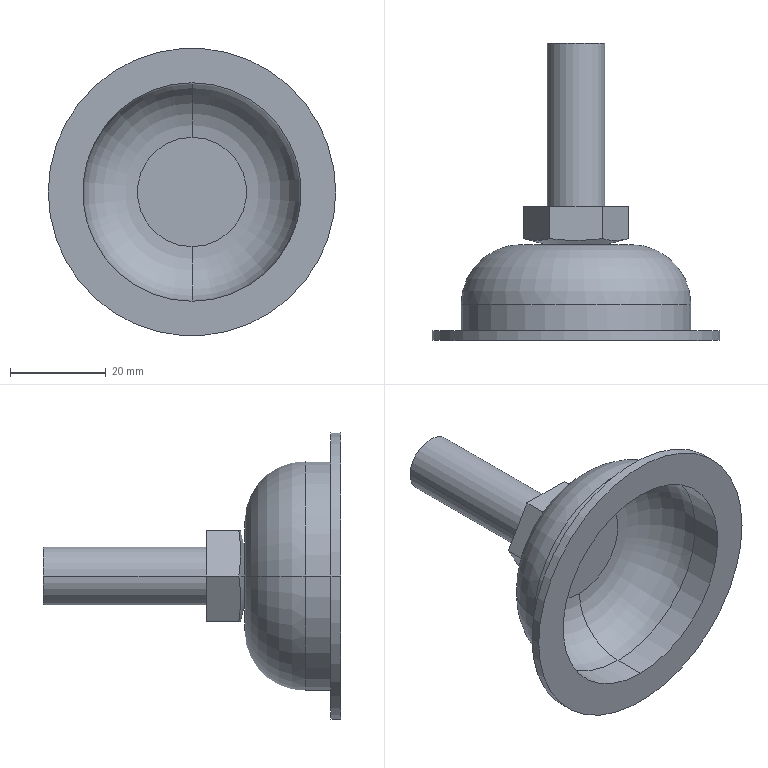Part | SolidWorks | features RefAxis 6, 3DProfileFeature 2, Revolution 2, Cut 1, ICE 1, RevCut 1 | 1 solid | 26 faces | box 60 x 62 x 60 mm | volume 14083 mm3 | plane 12 | cylinder 8 | torus 4 | cone 2 | commonest cylinder face diameters 12 x2 45.6 x2 48 x2 60 x2
STEP:
#1=CARTESIAN_POINT('',(0.,6.6,-22.8));
#2=VERTEX_POINT('',#1);
#3=CARTESIAN_POINT('',(0.,6.6,22.8));
#4=VERTEX_POINT('',#3);
#5=CARTESIAN_POINT('',(0.,6.6,0.));
#6=DIRECTION('',(0.,1.,0.));
#7=DIRECTION('',(0.,0.,1.));
#8=AXIS2_PLACEMENT_3D('',#5,#6,#7);
#9=CIRCLE('',#8,22.8);
#10=EDGE_CURVE('',#2,#4,#9,.T.);
#11=ORIENTED_EDGE('',*,*,#10,.F.);
#12=CARTESIAN_POINT('',(0.,18.,-11.4));
#13=VERTEX_POINT('',#12);
#14=CARTESIAN_POINT('',(0.,6.6,-11.4));
#15=DIRECTION('',(1.,0.,0.));
#16=DIRECTION('',(0.,0.,-1.));
#17=AXIS2_PLACEMENT_3D('',#14,#15,#16);
#18=CIRCLE('',#17,11.4);
#19=EDGE_CURVE('',#2,#13,#18,.T.);
#20=ORIENTED_EDGE('',*,*,#19,.T.);
#21=CARTESIAN_POINT('',(0.,18.,11.4));
#22=VERTEX_POINT('',#21);
#23=CARTESIAN_POINT('',(0.,18.,0.));
#24=DIRECTION('',(0.,1.,0.));
#25=DIRECTION('',(0.,0.,1.));
#26=AXIS2_PLACEMENT_3D('',#23,#24,#25);
#27=CIRCLE('',#26,11.4);
#28=EDGE_CURVE('',#13,#22,#27,.T.);
#29=ORIENTED_EDGE('',*,*,#28,.T.);
#30=CARTESIAN_POINT('',(0.,6.6,11.4));
#31=DIRECTION('',(-1.,0.,0.));
#32=DIRECTION('',(0.,0.,1.));
#33=AXIS2_PLACEMENT_3D('',#30,#31,#32);
#34=CIRCLE('',#33,11.4);
#35=EDGE_CURVE('',#4,#22,#34,.T.);
#36=ORIENTED_EDGE('',*,*,#35,.F.);
#37=EDGE_LOOP('',(#11,#20,#29,#36));
#38=FACE_OUTER_BOUND('',#37,.T.);
#39=CARTESIAN_POINT('',(0.,6.6,0.));
#40=DIRECTION('',(0.,1.,0.));
#41=DIRECTION('',(0.,0.,1.));
#42=AXIS2_PLACEMENT_3D('',#39,#40,#41);
#43=TOROIDAL_SURFACE('',#42,11.4,11.4);
#44=ADVANCED_FACE('',(#38),#43,.F.);
#45=CARTESIAN_POINT('',(0.,0.,22.8));
#46=VERTEX_POINT('',#45);
#47=CARTESIAN_POINT('',(0.,0.,-22.8));
#48=VERTEX_POINT('',#47);
#49=CARTESIAN_POINT('',(0.,0.,0.));
#50=DIRECTION('',(0.,-1.,0.));
#51=DIRECTION('',(-1.,0.,0.));
#52=AXIS2_PLACEMENT_3D('',#49,#50,#51);
#53=CIRCLE('',#52,22.8);
#54=EDGE_CURVE('',#46,#48,#53,.T.);
#55=ORIENTED_EDGE('',*,*,#54,.T.);
#56=CARTESIAN_POINT('',(0.,-1.,-22.8));
#57=DIRECTION('',(0.,1.,0.));
#58=VECTOR('',#57,1000.);
#59=LINE('',#56,#58);
#60=EDGE_CURVE('',#48,#2,#59,.T.);
#61=ORIENTED_EDGE('',*,*,#60,.T.);
#62=ORIENTED_EDGE('',*,*,#10,.T.);
#63=CARTESIAN_POINT('',(0.,-1.,22.8));
#64=DIRECTION('',(0.,1.,0.));
#65=VECTOR('',#64,1000.);
#66=LINE('',#63,#65);
#67=EDGE_CURVE('',#46,#4,#66,.T.);
#68=ORIENTED_EDGE('',*,*,#67,.F.);
#69=EDGE_LOOP('',(#55,#61,#62,#68));
#70=FACE_OUTER_BOUND('',#69,.T.);
#71=CARTESIAN_POINT('',(0.,-1.,0.));
#72=DIRECTION('',(0.,1.,0.));
#73=DIRECTION('',(0.,0.,1.));
#74=AXIS2_PLACEMENT_3D('',#71,#72,#73);
#75=CYLINDRICAL_SURFACE('',#74,22.8);
#76=ADVANCED_FACE('',(#70),#75,.F.);
#77=CARTESIAN_POINT('',(-30.,0.,0.));
#78=VERTEX_POINT('',#77);
#79=CARTESIAN_POINT('',(30.,0.,0.));
#80=VERTEX_POINT('',#79);
#81=CARTESIAN_POINT('',(0.,0.,0.));
#82=DIRECTION('',(0.,1.,0.));
#83=DIRECTION('',(-1.,0.,0.));
#84=AXIS2_PLACEMENT_3D('',#81,#82,#83);
#85=CIRCLE('',#84,30.);
#86=EDGE_CURVE('',#78,#80,#85,.T.);
#87=ORIENTED_EDGE('',*,*,#86,.T.);
#88=CARTESIAN_POINT('',(30.,2.,0.));
#89=VERTEX_POINT('',#88);
#90=CARTESIAN_POINT('',(30.,0.,0.));
#91=DIRECTION('',(0.,1.,0.));
#92=VECTOR('',#91,1000.);
#93=LINE('',#90,#92);
#94=EDGE_CURVE('',#80,#89,#93,.T.);
#95=ORIENTED_EDGE('',*,*,#94,.T.);
#96=CARTESIAN_POINT('',(-30.,2.,0.));
#97=VERTEX_POINT('',#96);
#98=CARTESIAN_POINT('',(0.,2.,0.));
#99=DIRECTION('',(0.,1.,0.));
#100=DIRECTION('',(-1.,0.,0.));
#101=AXIS2_PLACEMENT_3D('',#98,#99,#100);
#102=CIRCLE('',#101,30.);
#103=EDGE_CURVE('',#97,#89,#102,.T.);
#104=ORIENTED_EDGE('',*,*,#103,.F.);
#105=CARTESIAN_POINT('',(-30.,0.,0.));
#106=DIRECTION('',(0.,1.,0.));
#107=VECTOR('',#106,1000.);
#108=LINE('',#105,#107);
#109=EDGE_CURVE('',#78,#97,#108,.T.);
#110=ORIENTED_EDGE('',*,*,#109,.F.);
#111=EDGE_LOOP('',(#87,#95,#104,#110));
#112=FACE_OUTER_BOUND('',#111,.T.);
#113=CARTESIAN_POINT('',(0.,0.,0.));
#114=DIRECTION('',(0.,1.,0.));
#115=DIRECTION('',(-1.,0.,0.));
#116=AXIS2_PLACEMENT_3D('',#113,#114,#115);
#117=CYLINDRICAL_SURFACE('',#116,30.);
#118=ADVANCED_FACE('',(#112),#117,.T.);
#119=CARTESIAN_POINT('',(-24.,2.,0.));
#120=VERTEX_POINT('',#119);
#121=CARTESIAN_POINT('',(24.,2.,0.));
#122=VERTEX_POINT('',#121);
#123=CARTESIAN_POINT('',(0.,2.,0.));
#124=DIRECTION('',(0.,1.,0.));
#125=DIRECTION('',(-1.,0.,0.));
#126=AXIS2_PLACEMENT_3D('',#123,#124,#125);
#127=CIRCLE('',#126,24.);
#128=EDGE_CURVE('',#120,#122,#127,.T.);
#129=ORIENTED_EDGE('',*,*,#128,.T.);
#130=CARTESIAN_POINT('',(24.,7.4,0.));
#131=VERTEX_POINT('',#130);
#132=CARTESIAN_POINT('',(24.,0.,0.));
#133=DIRECTION('',(0.,1.,0.));
#134=VECTOR('',#133,1000.);
#135=LINE('',#132,#134);
#136=EDGE_CURVE('',#122,#131,#135,.T.);
#137=ORIENTED_EDGE('',*,*,#136,.T.);
#138=CARTESIAN_POINT('',(-24.,7.4,0.));
#139=VERTEX_POINT('',#138);
#140=CARTESIAN_POINT('',(0.,7.4,0.));
#141=DIRECTION('',(0.,1.,0.));
#142=DIRECTION('',(-1.,0.,0.));
#143=AXIS2_PLACEMENT_3D('',#140,#141,#142);
#144=CIRCLE('',#143,24.);
#145=EDGE_CURVE('',#139,#131,#144,.T.);
#146=ORIENTED_EDGE('',*,*,#145,.F.);
#147=CARTESIAN_POINT('',(-24.,0.,0.));
#148=DIRECTION('',(0.,1.,0.));
#149=VECTOR('',#148,1000.);
#150=LINE('',#147,#149);
#151=EDGE_CURVE('',#120,#139,#150,.T.);
#152=ORIENTED_EDGE('',*,*,#151,.F.);
#153=EDGE_LOOP('',(#129,#137,#146,#152));
#154=FACE_OUTER_BOUND('',#153,.T.);
#155=CARTESIAN_POINT('',(0.,0.,0.));
#156=DIRECTION('',(0.,1.,0.));
#157=DIRECTION('',(-1.,0.,0.));
#158=AXIS2_PLACEMENT_3D('',#155,#156,#157);
#159=CYLINDRICAL_SURFACE('',#158,24.);
#160=ADVANCED_FACE('',(#154),#159,.T.);
#161=ORIENTED_EDGE('',*,*,#145,.T.);
#162=CARTESIAN_POINT('',(11.4,20.,0.));
#163=VERTEX_POINT('',#162);
#164=CARTESIAN_POINT('',(11.4,7.4,0.));
#165=DIRECTION('',(0.,0.,1.));
#166=DIRECTION('',(1.,0.,0.));
#167=AXIS2_PLACEMENT_3D('',#164,#165,#166);
#168=CIRCLE('',#167,12.6);
#169=EDGE_CURVE('',#131,#163,#168,.T.);
#170=ORIENTED_EDGE('',*,*,#169,.T.);
#171=CARTESIAN_POINT('',(-11.4,20.,0.));
#172=VERTEX_POINT('',#171);
#173=CARTESIAN_POINT('',(0.,20.,0.));
#174=DIRECTION('',(0.,1.,0.));
#175=DIRECTION('',(-1.,0.,0.));
#176=AXIS2_PLACEMENT_3D('',#173,#174,#175);
#177=CIRCLE('',#176,11.4);
#178=EDGE_CURVE('',#172,#163,#177,.T.);
#179=ORIENTED_EDGE('',*,*,#178,.F.);
#180=CARTESIAN_POINT('',(-11.4,7.4,0.));
#181=DIRECTION('',(0.,0.,-1.));
#182=DIRECTION('',(-1.,0.,0.));
#183=AXIS2_PLACEMENT_3D('',#180,#181,#182);
#184=CIRCLE('',#183,12.6);
#185=EDGE_CURVE('',#139,#172,#184,.T.);
#186=ORIENTED_EDGE('',*,*,#185,.F.);
#187=EDGE_LOOP('',(#161,#170,#179,#186));
#188=FACE_OUTER_BOUND('',#187,.T.);
#189=CARTESIAN_POINT('',(0.,7.4,0.));
#190=DIRECTION('',(0.,1.,0.));
#191=DIRECTION('',(-1.,0.,0.));
#192=AXIS2_PLACEMENT_3D('',#189,#190,#191);
#193=TOROIDAL_SURFACE('',#192,11.4,12.6);
#194=ADVANCED_FACE('',(#188),#193,.T.);
#195=CARTESIAN_POINT('',(-6.,20.,0.));
#196=VERTEX_POINT('',#195);
#197=CARTESIAN_POINT('',(6.,20.,0.));
#198=VERTEX_POINT('',#197);
#199=CARTESIAN_POINT('',(0.,20.,0.));
#200=DIRECTION('',(0.,1.,0.));
#201=DIRECTION('',(-1.,0.,0.));
#202=AXIS2_PLACEMENT_3D('',#199,#200,#201);
#203=CIRCLE('',#202,6.);
#204=EDGE_CURVE('',#196,#198,#203,.T.);
#205=ORIENTED_EDGE('',*,*,#204,.T.);
#206=CARTESIAN_POINT('',(10.97,21.236,0.));
#207=VERTEX_POINT('',#206);
#208=CARTESIAN_POINT('',(6.,20.,0.));
#209=DIRECTION('',(0.9704,0.2414,0.));
#210=VECTOR('',#209,1000.);
#211=LINE('',#208,#210);
#212=EDGE_CURVE('',#198,#207,#211,.T.);
#213=ORIENTED_EDGE('',*,*,#212,.T.);
#214=CARTESIAN_POINT('',(5.485,21.236,9.5));
#215=VERTEX_POINT('',#214);
#216=CARTESIAN_POINT('',(10.97,21.236,0.));
#217=CARTESIAN_POINT('',(10.513,21.123,0.7917));
#218=CARTESIAN_POINT('',(10.056,21.03,1.583));
#219=CARTESIAN_POINT('',(9.141,20.904,3.167));
#220=CARTESIAN_POINT('',(8.227,20.837,4.75));
#221=CARTESIAN_POINT('',(7.313,20.904,6.333));
#222=CARTESIAN_POINT('',(6.399,21.03,7.917));
#223=CARTESIAN_POINT('',(5.942,21.123,8.708));
#224=CARTESIAN_POINT('',(5.485,21.236,9.5));
#225=B_SPLINE_CURVE_WITH_KNOTS('',3,(#216,#217,#218,#219,#220,#221,#222,#223,#224),.UNSPECIFIED.,.F.,.F.,(4,2,1,2,4),(0.000000231,0.002743,0.005485,0.008227,0.01097),.UNSPECIFIED.);
#226=EDGE_CURVE('',#207,#215,#225,.T.);
#227=ORIENTED_EDGE('',*,*,#226,.T.);
#228=CARTESIAN_POINT('',(-5.485,21.236,9.5));
#229=VERTEX_POINT('',#228);
#230=CARTESIAN_POINT('',(5.485,21.236,9.5));
#231=CARTESIAN_POINT('',(3.662,21.01,9.5));
#232=CARTESIAN_POINT('',(1.837,20.871,9.5));
#233=CARTESIAN_POINT('',(-0.9062,20.871,9.5));
#234=CARTESIAN_POINT('',(-1.822,20.904,9.5));
#235=CARTESIAN_POINT('',(-3.654,21.03,9.5));
#236=CARTESIAN_POINT('',(-4.572,21.123,9.5));
#237=CARTESIAN_POINT('',(-5.485,21.236,9.5));
#238=B_SPLINE_CURVE_WITH_KNOTS('',3,(#230,#231,#232,#233,#234,#235,#236,#237),.UNSPECIFIED.,.F.,.F.,(4,2,2,4),(0.02128,0.02679,0.02955,0.0323),.UNSPECIFIED.);
#239=EDGE_CURVE('',#215,#229,#238,.T.);
#240=ORIENTED_EDGE('',*,*,#239,.T.);
#241=CARTESIAN_POINT('',(-10.97,21.236,0.));
#242=VERTEX_POINT('',#241);
#243=CARTESIAN_POINT('',(-5.485,21.236,9.5));
#244=CARTESIAN_POINT('',(-5.942,21.123,8.708));
#245=CARTESIAN_POINT('',(-6.399,21.03,7.917));
#246=CARTESIAN_POINT('',(-7.313,20.904,6.333));
#247=CARTESIAN_POINT('',(-8.227,20.837,4.75));
#248=CARTESIAN_POINT('',(-9.141,20.904,3.167));
#249=CARTESIAN_POINT('',(-10.056,21.03,1.583));
#250=CARTESIAN_POINT('',(-10.513,21.123,0.7917));
#251=CARTESIAN_POINT('',(-10.97,21.236,0.));
#252=B_SPLINE_CURVE_WITH_KNOTS('',3,(#243,#244,#245,#246,#247,#248,#249,#250,#251),.UNSPECIFIED.,.F.,.F.,(4,2,1,2,4),(0.000000231,0.002743,0.005485,0.008227,0.01097),.UNSPECIFIED.);
#253=EDGE_CURVE('',#229,#242,#252,.T.);
#254=ORIENTED_EDGE('',*,*,#253,.T.);
#255=CARTESIAN_POINT('',(-6.,20.,0.));
#256=DIRECTION('',(-0.9704,0.2414,0.));
#257=VECTOR('',#256,1000.);
#258=LINE('',#255,#257);
#259=EDGE_CURVE('',#196,#242,#258,.T.);
#260=ORIENTED_EDGE('',*,*,#259,.F.);
#261=EDGE_LOOP('',(#205,#213,#227,#240,#254,#260));
#262=FACE_OUTER_BOUND('',#261,.T.);
#263=CARTESIAN_POINT('',(0.,20.,0.));
#264=DIRECTION('',(0.,1.,0.));
#265=DIRECTION('',(-1.,0.,0.));
#266=AXIS2_PLACEMENT_3D('',#263,#264,#265);
#267=CONICAL_SURFACE('',#266,6.,1.327);
#268=ADVANCED_FACE('',(#262),#267,.T.);
#269=CARTESIAN_POINT('',(-6.,28.,0.));
#270=VERTEX_POINT('',#269);
#271=CARTESIAN_POINT('',(6.,28.,0.));
#272=VERTEX_POINT('',#271);
#273=CARTESIAN_POINT('',(0.,28.,0.));
#274=DIRECTION('',(0.,1.,0.));
#275=DIRECTION('',(1.,0.,0.));
#276=AXIS2_PLACEMENT_3D('',#273,#274,#275);
#277=CIRCLE('',#276,6.);
#278=EDGE_CURVE('',#270,#272,#277,.T.);
#279=ORIENTED_EDGE('',*,*,#278,.T.);
#280=CARTESIAN_POINT('',(6.,62.,0.));
#281=VERTEX_POINT('',#280);
#282=CARTESIAN_POINT('',(6.,28.,0.));
#283=DIRECTION('',(0.,1.,0.));
#284=VECTOR('',#283,1000.);
#285=LINE('',#282,#284);
#286=EDGE_CURVE('',#272,#281,#285,.T.);
#287=ORIENTED_EDGE('',*,*,#286,.T.);
#288=CARTESIAN_POINT('',(-6.,62.,0.));
#289=VERTEX_POINT('',#288);
#290=CARTESIAN_POINT('',(0.,62.,0.));
#291=DIRECTION('',(0.,1.,0.));
#292=DIRECTION('',(-1.,0.,0.));
#293=AXIS2_PLACEMENT_3D('',#290,#291,#292);
#294=CIRCLE('',#293,6.);
#295=EDGE_CURVE('',#289,#281,#294,.T.);
#296=ORIENTED_EDGE('',*,*,#295,.F.);
#297=CARTESIAN_POINT('',(-6.,28.,0.));
#298=DIRECTION('',(0.,1.,0.));
#299=VECTOR('',#298,1000.);
#300=LINE('',#297,#299);
#301=EDGE_CURVE('',#270,#289,#300,.T.);
#302=ORIENTED_EDGE('',*,*,#301,.F.);
#303=EDGE_LOOP('',(#279,#287,#296,#302));
#304=FACE_OUTER_BOUND('',#303,.T.);
#305=CARTESIAN_POINT('',(0.,28.,0.));
#306=DIRECTION('',(0.,1.,0.));
#307=DIRECTION('',(-1.,0.,0.));
#308=AXIS2_PLACEMENT_3D('',#305,#306,#307);
#309=CYLINDRICAL_SURFACE('',#308,6.);
#310=ADVANCED_FACE('',(#304),#309,.T.);
#311=ORIENTED_EDGE('',*,*,#286,.F.);
#312=CARTESIAN_POINT('',(0.,28.,0.));
#313=DIRECTION('',(0.,1.,0.));
#314=DIRECTION('',(1.,0.,0.));
#315=AXIS2_PLACEMENT_3D('',#312,#313,#314);
#316=CIRCLE('',#315,6.);
#317=EDGE_CURVE('',#272,#270,#316,.T.);
#318=ORIENTED_EDGE('',*,*,#317,.T.);
#319=ORIENTED_EDGE('',*,*,#301,.T.);
#320=CARTESIAN_POINT('',(0.,62.,0.));
#321=DIRECTION('',(0.,1.,0.));
#322=DIRECTION('',(-1.,0.,0.));
#323=AXIS2_PLACEMENT_3D('',#320,#321,#322);
#324=CIRCLE('',#323,6.);
#325=EDGE_CURVE('',#281,#289,#324,.T.);
#326=ORIENTED_EDGE('',*,*,#325,.F.);
#327=EDGE_LOOP('',(#311,#318,#319,#326));
#328=FACE_OUTER_BOUND('',#327,.T.);
#329=CARTESIAN_POINT('',(0.,28.,0.));
#330=DIRECTION('',(0.,1.,0.));
#331=DIRECTION('',(-1.,0.,0.));
#332=AXIS2_PLACEMENT_3D('',#329,#330,#331);
#333=CYLINDRICAL_SURFACE('',#332,6.);
#334=ADVANCED_FACE('',(#328),#333,.T.);
#335=ORIENTED_EDGE('',*,*,#86,.F.);
#336=CARTESIAN_POINT('',(0.,0.,0.));
#337=DIRECTION('',(0.,1.,0.));
#338=DIRECTION('',(-1.,0.,0.));
#339=AXIS2_PLACEMENT_3D('',#336,#337,#338);
#340=CIRCLE('',#339,30.);
#341=EDGE_CURVE('',#80,#78,#340,.T.);
#342=ORIENTED_EDGE('',*,*,#341,.F.);
#343=EDGE_LOOP('',(#335,#342));
#344=FACE_OUTER_BOUND('',#343,.T.);
#345=ORIENTED_EDGE('',*,*,#54,.F.);
#346=CARTESIAN_POINT('',(0.,0.,0.));
#347=DIRECTION('',(0.,-1.,0.));
#348=DIRECTION('',(-1.,0.,0.));
#349=AXIS2_PLACEMENT_3D('',#346,#347,#348);
#350=CIRCLE('',#349,22.8);
#351=EDGE_CURVE('',#48,#46,#350,.T.);
#352=ORIENTED_EDGE('',*,*,#351,.F.);
#353=EDGE_LOOP('',(#345,#352));
#354=FACE_BOUND('',#353,.T.);
#355=CARTESIAN_POINT('',(30.,0.,0.));
#356=DIRECTION('',(0.,1.,0.));
#357=DIRECTION('',(-1.,0.,0.));
#358=AXIS2_PLACEMENT_3D('',#355,#356,#357);
#359=PLANE('',#358);
#360=ADVANCED_FACE('',(#344,#354),#359,.F.);
#361=ORIENTED_EDGE('',*,*,#212,.F.);
#362=CARTESIAN_POINT('',(0.,20.,0.));
#363=DIRECTION('',(0.,1.,0.));
#364=DIRECTION('',(-1.,0.,0.));
#365=AXIS2_PLACEMENT_3D('',#362,#363,#364);
#366=CIRCLE('',#365,6.);
#367=EDGE_CURVE('',#198,#196,#366,.T.);
#368=ORIENTED_EDGE('',*,*,#367,.T.);
#369=ORIENTED_EDGE('',*,*,#259,.T.);
#370=CARTESIAN_POINT('',(-5.485,21.236,-9.5));
#371=VERTEX_POINT('',#370);
#372=CARTESIAN_POINT('',(-10.97,21.236,0.));
#373=CARTESIAN_POINT('',(-10.513,21.123,-0.7917));
#374=CARTESIAN_POINT('',(-10.056,21.03,-1.583));
#375=CARTESIAN_POINT('',(-9.141,20.904,-3.167));
#376=CARTESIAN_POINT('',(-8.227,20.837,-4.75));
#377=CARTESIAN_POINT('',(-7.313,20.904,-6.333));
#378=CARTESIAN_POINT('',(-6.399,21.03,-7.917));
#379=CARTESIAN_POINT('',(-5.942,21.123,-8.708));
#380=CARTESIAN_POINT('',(-5.485,21.236,-9.5));
#381=B_SPLINE_CURVE_WITH_KNOTS('',3,(#372,#373,#374,#375,#376,#377,#378,#379,#380),.UNSPECIFIED.,.F.,.F.,(4,2,1,2,4),(0.000000231,0.002743,0.005485,0.008227,0.01097),.UNSPECIFIED.);
#382=EDGE_CURVE('',#242,#371,#381,.T.);
#383=ORIENTED_EDGE('',*,*,#382,.T.);
#384=CARTESIAN_POINT('',(5.485,21.236,-9.5));
#385=VERTEX_POINT('',#384);
#386=CARTESIAN_POINT('',(-5.485,21.236,-9.5));
#387=CARTESIAN_POINT('',(-4.572,21.123,-9.5));
#388=CARTESIAN_POINT('',(-3.654,21.03,-9.5));
#389=CARTESIAN_POINT('',(-1.822,20.904,-9.5));
#390=CARTESIAN_POINT('',(-0.9062,20.871,-9.5));
#391=CARTESIAN_POINT('',(1.837,20.871,-9.5));
#392=CARTESIAN_POINT('',(3.662,21.01,-9.5));
#393=CARTESIAN_POINT('',(5.485,21.236,-9.5));
#394=B_SPLINE_CURVE_WITH_KNOTS('',3,(#386,#387,#388,#389,#390,#391,#392,#393),.UNSPECIFIED.,.F.,.F.,(4,2,2,4),(0.009106,0.01186,0.01462,0.02014),.UNSPECIFIED.);
#395=EDGE_CURVE('',#371,#385,#394,.T.);
#396=ORIENTED_EDGE('',*,*,#395,.T.);
#397=CARTESIAN_POINT('',(5.485,21.236,-9.5));
#398=CARTESIAN_POINT('',(5.942,21.123,-8.708));
#399=CARTESIAN_POINT('',(6.399,21.03,-7.917));
#400=CARTESIAN_POINT('',(7.313,20.904,-6.333));
#401=CARTESIAN_POINT('',(8.227,20.837,-4.75));
#402=CARTESIAN_POINT('',(9.141,20.904,-3.167));
#403=CARTESIAN_POINT('',(10.056,21.03,-1.583));
#404=CARTESIAN_POINT('',(10.513,21.123,-0.7917));
#405=CARTESIAN_POINT('',(10.97,21.236,0.));
#406=B_SPLINE_CURVE_WITH_KNOTS('',3,(#397,#398,#399,#400,#401,#402,#403,#404,#405),.UNSPECIFIED.,.F.,.F.,(4,2,1,2,4),(0.000000231,0.002743,0.005485,0.008227,0.01097),.UNSPECIFIED.);
#407=EDGE_CURVE('',#385,#207,#406,.T.);
#408=ORIENTED_EDGE('',*,*,#407,.T.);
#409=EDGE_LOOP('',(#361,#368,#369,#383,#396,#408));
#410=FACE_OUTER_BOUND('',#409,.T.);
#411=CARTESIAN_POINT('',(0.,20.,0.));
#412=DIRECTION('',(0.,1.,0.));
#413=DIRECTION('',(-1.,0.,0.));
#414=AXIS2_PLACEMENT_3D('',#411,#412,#413);
#415=CONICAL_SURFACE('',#414,6.,1.327);
#416=ADVANCED_FACE('',(#410),#415,.T.);
#417=ORIENTED_EDGE('',*,*,#204,.F.);
#418=ORIENTED_EDGE('',*,*,#367,.F.);
#419=EDGE_LOOP('',(#417,#418));
#420=FACE_BOUND('',#419,.T.);
#421=ORIENTED_EDGE('',*,*,#178,.T.);
#422=CARTESIAN_POINT('',(0.,20.,0.));
#423=DIRECTION('',(0.,1.,0.));
#424=DIRECTION('',(-1.,0.,0.));
#425=AXIS2_PLACEMENT_3D('',#422,#423,#424);
#426=CIRCLE('',#425,11.4);
#427=EDGE_CURVE('',#163,#172,#426,.T.);
#428=ORIENTED_EDGE('',*,*,#427,.T.);
#429=EDGE_LOOP('',(#421,#428));
#430=FACE_OUTER_BOUND('',#429,.T.);
#431=CARTESIAN_POINT('',(6.,20.,0.));
#432=DIRECTION('',(0.,-1.,0.));
#433=DIRECTION('',(1.,0.,0.));
#434=AXIS2_PLACEMENT_3D('',#431,#432,#433);
#435=PLANE('',#434);
#436=ADVANCED_FACE('',(#420,#430),#435,.F.);
#437=ORIENTED_EDGE('',*,*,#169,.F.);
#438=CARTESIAN_POINT('',(0.,7.4,0.));
#439=DIRECTION('',(0.,1.,0.));
#440=DIRECTION('',(-1.,0.,0.));
#441=AXIS2_PLACEMENT_3D('',#438,#439,#440);
#442=CIRCLE('',#441,24.);
#443=EDGE_CURVE('',#131,#139,#442,.T.);
#444=ORIENTED_EDGE('',*,*,#443,.T.);
#445=ORIENTED_EDGE('',*,*,#185,.T.);
#446=ORIENTED_EDGE('',*,*,#427,.F.);
#447=EDGE_LOOP('',(#437,#444,#445,#446));
#448=FACE_OUTER_BOUND('',#447,.T.);
#449=CARTESIAN_POINT('',(0.,7.4,0.));
#450=DIRECTION('',(0.,1.,0.));
#451=DIRECTION('',(-1.,0.,0.));
#452=AXIS2_PLACEMENT_3D('',#449,#450,#451);
#453=TOROIDAL_SURFACE('',#452,11.4,12.6);
#454=ADVANCED_FACE('',(#448),#453,.T.);
#455=ORIENTED_EDGE('',*,*,#136,.F.);
#456=CARTESIAN_POINT('',(0.,2.,0.));
#457=DIRECTION('',(0.,1.,0.));
#458=DIRECTION('',(-1.,0.,0.));
#459=AXIS2_PLACEMENT_3D('',#456,#457,#458);
#460=CIRCLE('',#459,24.);
#461=EDGE_CURVE('',#122,#120,#460,.T.);
#462=ORIENTED_EDGE('',*,*,#461,.T.);
#463=ORIENTED_EDGE('',*,*,#151,.T.);
#464=ORIENTED_EDGE('',*,*,#443,.F.);
#465=EDGE_LOOP('',(#455,#462,#463,#464));
#466=FACE_OUTER_BOUND('',#465,.T.);
#467=CARTESIAN_POINT('',(0.,0.,0.));
#468=DIRECTION('',(0.,1.,0.));
#469=DIRECTION('',(-1.,0.,0.));
#470=AXIS2_PLACEMENT_3D('',#467,#468,#469);
#471=CYLINDRICAL_SURFACE('',#470,24.);
#472=ADVANCED_FACE('',(#466),#471,.T.);
#473=ORIENTED_EDGE('',*,*,#128,.F.);
#474=ORIENTED_EDGE('',*,*,#461,.F.);
#475=EDGE_LOOP('',(#473,#474));
#476=FACE_BOUND('',#475,.T.);
#477=ORIENTED_EDGE('',*,*,#103,.T.);
#478=CARTESIAN_POINT('',(0.,2.,0.));
#479=DIRECTION('',(0.,1.,0.));
#480=DIRECTION('',(-1.,0.,0.));
#481=AXIS2_PLACEMENT_3D('',#478,#479,#480);
#482=CIRCLE('',#481,30.);
#483=EDGE_CURVE('',#89,#97,#482,.T.);
#484=ORIENTED_EDGE('',*,*,#483,.T.);
#485=EDGE_LOOP('',(#477,#484));
#486=FACE_OUTER_BOUND('',#485,.T.);
#487=CARTESIAN_POINT('',(24.,2.,0.));
#488=DIRECTION('',(0.,-1.,0.));
#489=DIRECTION('',(1.,0.,0.));
#490=AXIS2_PLACEMENT_3D('',#487,#488,#489);
#491=PLANE('',#490);
#492=ADVANCED_FACE('',(#476,#486),#491,.F.);
#493=ORIENTED_EDGE('',*,*,#94,.F.);
#494=ORIENTED_EDGE('',*,*,#341,.T.);
#495=ORIENTED_EDGE('',*,*,#109,.T.);
#496=ORIENTED_EDGE('',*,*,#483,.F.);
#497=EDGE_LOOP('',(#493,#494,#495,#496));
#498=FACE_OUTER_BOUND('',#497,.T.);
#499=CARTESIAN_POINT('',(0.,0.,0.));
#500=DIRECTION('',(0.,1.,0.));
#501=DIRECTION('',(-1.,0.,0.));
#502=AXIS2_PLACEMENT_3D('',#499,#500,#501);
#503=CYLINDRICAL_SURFACE('',#502,30.);
#504=ADVANCED_FACE('',(#498),#503,.T.);
#505=CARTESIAN_POINT('',(-5.485,28.,-9.5));
#506=VERTEX_POINT('',#505);
#507=CARTESIAN_POINT('',(-5.485,29.,-9.5));
#508=DIRECTION('',(0.,-1.,0.));
#509=VECTOR('',#508,1000.);
#510=LINE('',#507,#509);
#511=EDGE_CURVE('',#506,#371,#510,.T.);
#512=ORIENTED_EDGE('',*,*,#511,.T.);
#513=ORIENTED_EDGE('',*,*,#382,.F.);
#514=CARTESIAN_POINT('',(-10.97,28.,0.));
#515=VERTEX_POINT('',#514);
#516=CARTESIAN_POINT('',(-10.97,29.,0.));
#517=DIRECTION('',(0.,-1.,0.));
#518=VECTOR('',#517,1000.);
#519=LINE('',#516,#518);
#520=EDGE_CURVE('',#515,#242,#519,.T.);
#521=ORIENTED_EDGE('',*,*,#520,.F.);
#522=CARTESIAN_POINT('',(-8.227,28.,-4.75));
#523=DIRECTION('',(-0.5,0.,0.866));
#524=VECTOR('',#523,1000.);
#525=LINE('',#522,#524);
#526=EDGE_CURVE('',#506,#515,#525,.T.);
#527=ORIENTED_EDGE('',*,*,#526,.F.);
#528=EDGE_LOOP('',(#512,#513,#521,#527));
#529=FACE_OUTER_BOUND('',#528,.T.);
#530=CARTESIAN_POINT('',(-5.485,29.,-9.5));
#531=DIRECTION('',(0.866,0.,0.5));
#532=DIRECTION('',(0.5,0.,-0.866));
#533=AXIS2_PLACEMENT_3D('',#530,#531,#532);
#534=PLANE('',#533);
#535=ADVANCED_FACE('',(#529),#534,.F.);
#536=ORIENTED_EDGE('',*,*,#520,.T.);
#537=ORIENTED_EDGE('',*,*,#253,.F.);
#538=CARTESIAN_POINT('',(-5.485,28.,9.5));
#539=VERTEX_POINT('',#538);
#540=CARTESIAN_POINT('',(-5.485,29.,9.5));
#541=DIRECTION('',(0.,-1.,0.));
#542=VECTOR('',#541,1000.);
#543=LINE('',#540,#542);
#544=EDGE_CURVE('',#539,#229,#543,.T.);
#545=ORIENTED_EDGE('',*,*,#544,.F.);
#546=CARTESIAN_POINT('',(-8.227,28.,4.75));
#547=DIRECTION('',(0.5,0.,0.866));
#548=VECTOR('',#547,1000.);
#549=LINE('',#546,#548);
#550=EDGE_CURVE('',#515,#539,#549,.T.);
#551=ORIENTED_EDGE('',*,*,#550,.F.);
#552=EDGE_LOOP('',(#536,#537,#545,#551));
#553=FACE_OUTER_BOUND('',#552,.T.);
#554=CARTESIAN_POINT('',(-10.97,29.,0.));
#555=DIRECTION('',(0.866,0.,-0.5));
#556=DIRECTION('',(-0.5,0.,-0.866));
#557=AXIS2_PLACEMENT_3D('',#554,#555,#556);
#558=PLANE('',#557);
#559=ADVANCED_FACE('',(#553),#558,.F.);
#560=ORIENTED_EDGE('',*,*,#544,.T.);
#561=ORIENTED_EDGE('',*,*,#239,.F.);
#562=CARTESIAN_POINT('',(5.485,28.,9.5));
#563=VERTEX_POINT('',#562);
#564=CARTESIAN_POINT('',(5.485,29.,9.5));
#565=DIRECTION('',(0.,-1.,0.));
#566=VECTOR('',#565,1000.);
#567=LINE('',#564,#566);
#568=EDGE_CURVE('',#563,#215,#567,.T.);
#569=ORIENTED_EDGE('',*,*,#568,.F.);
#570=CARTESIAN_POINT('',(0.,28.,9.5));
#571=DIRECTION('',(1.,0.,0.));
#572=VECTOR('',#571,1000.);
#573=LINE('',#570,#572);
#574=EDGE_CURVE('',#539,#563,#573,.T.);
#575=ORIENTED_EDGE('',*,*,#574,.F.);
#576=EDGE_LOOP('',(#560,#561,#569,#575));
#577=FACE_OUTER_BOUND('',#576,.T.);
#578=CARTESIAN_POINT('',(-5.485,29.,9.5));
#579=DIRECTION('',(0.,0.,-1.));
#580=DIRECTION('',(-1.,0.,0.));
#581=AXIS2_PLACEMENT_3D('',#578,#579,#580);
#582=PLANE('',#581);
#583=ADVANCED_FACE('',(#577),#582,.F.);
#584=ORIENTED_EDGE('',*,*,#568,.T.);
#585=ORIENTED_EDGE('',*,*,#226,.F.);
#586=CARTESIAN_POINT('',(10.97,28.,0.));
#587=VERTEX_POINT('',#586);
#588=CARTESIAN_POINT('',(10.97,29.,0.));
#589=DIRECTION('',(0.,-1.,0.));
#590=VECTOR('',#589,1000.);
#591=LINE('',#588,#590);
#592=EDGE_CURVE('',#587,#207,#591,.T.);
#593=ORIENTED_EDGE('',*,*,#592,.F.);
#594=CARTESIAN_POINT('',(8.227,28.,4.75));
#595=DIRECTION('',(0.5,0.,-0.866));
#596=VECTOR('',#595,1000.);
#597=LINE('',#594,#596);
#598=EDGE_CURVE('',#563,#587,#597,.T.);
#599=ORIENTED_EDGE('',*,*,#598,.F.);
#600=EDGE_LOOP('',(#584,#585,#593,#599));
#601=FACE_OUTER_BOUND('',#600,.T.);
#602=CARTESIAN_POINT('',(5.485,29.,9.5));
#603=DIRECTION('',(-0.866,0.,-0.5));
#604=DIRECTION('',(-0.5,0.,0.866));
#605=AXIS2_PLACEMENT_3D('',#602,#603,#604);
#606=PLANE('',#605);
#607=ADVANCED_FACE('',(#601),#606,.F.);
#608=ORIENTED_EDGE('',*,*,#592,.T.);
#609=ORIENTED_EDGE('',*,*,#407,.F.);
#610=CARTESIAN_POINT('',(5.485,28.,-9.5));
#611=VERTEX_POINT('',#610);
#612=CARTESIAN_POINT('',(5.485,29.,-9.5));
#613=DIRECTION('',(0.,-1.,0.));
#614=VECTOR('',#613,1000.);
#615=LINE('',#612,#614);
#616=EDGE_CURVE('',#611,#385,#615,.T.);
#617=ORIENTED_EDGE('',*,*,#616,.F.);
#618=CARTESIAN_POINT('',(8.227,28.,-4.75));
#619=DIRECTION('',(-0.5,0.,-0.866));
#620=VECTOR('',#619,1000.);
#621=LINE('',#618,#620);
#622=EDGE_CURVE('',#587,#611,#621,.T.);
#623=ORIENTED_EDGE('',*,*,#622,.F.);
#624=EDGE_LOOP('',(#608,#609,#617,#623));
#625=FACE_OUTER_BOUND('',#624,.T.);
#626=CARTESIAN_POINT('',(10.97,29.,0.));
#627=DIRECTION('',(-0.866,0.,0.5));
#628=DIRECTION('',(0.5,0.,0.866));
#629=AXIS2_PLACEMENT_3D('',#626,#627,#628);
#630=PLANE('',#629);
#631=ADVANCED_FACE('',(#625),#630,.F.);
#632=ORIENTED_EDGE('',*,*,#616,.T.);
#633=ORIENTED_EDGE('',*,*,#395,.F.);
#634=ORIENTED_EDGE('',*,*,#511,.F.);
#635=CARTESIAN_POINT('',(0.,28.,-9.5));
#636=DIRECTION('',(-1.,0.,0.));
#637=VECTOR('',#636,1000.);
#638=LINE('',#635,#637);
#639=EDGE_CURVE('',#611,#506,#638,.T.);
#640=ORIENTED_EDGE('',*,*,#639,.F.);
#641=EDGE_LOOP('',(#632,#633,#634,#640));
#642=FACE_OUTER_BOUND('',#641,.T.);
#643=CARTESIAN_POINT('',(5.485,29.,-9.5));
#644=DIRECTION('',(0.,0.,1.));
#645=DIRECTION('',(1.,0.,0.));
#646=AXIS2_PLACEMENT_3D('',#643,#644,#645);
#647=PLANE('',#646);
#648=ADVANCED_FACE('',(#642),#647,.F.);
#649=ORIENTED_EDGE('',*,*,#639,.T.);
#650=ORIENTED_EDGE('',*,*,#526,.T.);
#651=ORIENTED_EDGE('',*,*,#550,.T.);
#652=ORIENTED_EDGE('',*,*,#574,.T.);
#653=ORIENTED_EDGE('',*,*,#598,.T.);
#654=ORIENTED_EDGE('',*,*,#622,.T.);
#655=EDGE_LOOP('',(#649,#650,#651,#652,#653,#654));
#656=FACE_OUTER_BOUND('',#655,.T.);
#657=ORIENTED_EDGE('',*,*,#278,.F.);
#658=ORIENTED_EDGE('',*,*,#317,.F.);
#659=EDGE_LOOP('',(#657,#658));
#660=FACE_BOUND('',#659,.T.);
#661=CARTESIAN_POINT('',(0.,28.,0.));
#662=DIRECTION('',(0.,-1.,0.));
#663=DIRECTION('',(1.,0.,0.));
#664=AXIS2_PLACEMENT_3D('',#661,#662,#663);
#665=PLANE('',#664);
#666=ADVANCED_FACE('',(#656,#660),#665,.F.);
#667=ORIENTED_EDGE('',*,*,#60,.F.);
#668=ORIENTED_EDGE('',*,*,#351,.T.);
#669=ORIENTED_EDGE('',*,*,#67,.T.);
#670=CARTESIAN_POINT('',(0.,6.6,0.));
#671=DIRECTION('',(0.,1.,0.));
#672=DIRECTION('',(0.,0.,1.));
#673=AXIS2_PLACEMENT_3D('',#670,#671,#672);
#674=CIRCLE('',#673,22.8);
#675=EDGE_CURVE('',#4,#2,#674,.T.);
#676=ORIENTED_EDGE('',*,*,#675,.T.);
#677=EDGE_LOOP('',(#667,#668,#669,#676));
#678=FACE_OUTER_BOUND('',#677,.T.);
#679=CARTESIAN_POINT('',(0.,-1.,0.));
#680=DIRECTION('',(0.,1.,0.));
#681=DIRECTION('',(0.,0.,1.));
#682=AXIS2_PLACEMENT_3D('',#679,#680,#681);
#683=CYLINDRICAL_SURFACE('',#682,22.8);
#684=ADVANCED_FACE('',(#678),#683,.F.);
#685=CARTESIAN_POINT('',(0.,18.,0.));
#686=DIRECTION('',(0.,1.,0.));
#687=DIRECTION('',(0.,0.,1.));
#688=AXIS2_PLACEMENT_3D('',#685,#686,#687);
#689=CIRCLE('',#688,11.4);
#690=EDGE_CURVE('',#22,#13,#689,.T.);
#691=ORIENTED_EDGE('',*,*,#690,.F.);
#692=ORIENTED_EDGE('',*,*,#28,.F.);
#693=EDGE_LOOP('',(#691,#692));
#694=FACE_OUTER_BOUND('',#693,.T.);
#695=CARTESIAN_POINT('',(0.,18.,0.));
#696=DIRECTION('',(0.,-1.,0.));
#697=DIRECTION('',(0.,0.,-1.));
#698=AXIS2_PLACEMENT_3D('',#695,#696,#697);
#699=PLANE('',#698);
#700=ADVANCED_FACE('',(#694),#699,.T.);
#701=ORIENTED_EDGE('',*,*,#19,.F.);
#702=ORIENTED_EDGE('',*,*,#675,.F.);
#703=ORIENTED_EDGE('',*,*,#35,.T.);
#704=ORIENTED_EDGE('',*,*,#690,.T.);
#705=EDGE_LOOP('',(#701,#702,#703,#704));
#706=FACE_OUTER_BOUND('',#705,.T.);
#707=CARTESIAN_POINT('',(0.,6.6,0.));
#708=DIRECTION('',(0.,1.,0.));
#709=DIRECTION('',(0.,0.,1.));
#710=AXIS2_PLACEMENT_3D('',#707,#708,#709);
#711=TOROIDAL_SURFACE('',#710,11.4,11.4);
#712=ADVANCED_FACE('',(#706),#711,.F.);
#713=ORIENTED_EDGE('',*,*,#295,.T.);
#714=ORIENTED_EDGE('',*,*,#325,.T.);
#715=EDGE_LOOP('',(#713,#714));
#716=FACE_OUTER_BOUND('',#715,.T.);
#717=CARTESIAN_POINT('',(0.,62.,0.));
#718=DIRECTION('',(0.,1.,0.));
#719=DIRECTION('',(-1.,0.,0.));
#720=AXIS2_PLACEMENT_3D('',#717,#718,#719);
#721=PLANE('',#720);
#722=ADVANCED_FACE('',(#716),#721,.T.);
#723=CLOSED_SHELL('',(#44,#76,#118,#160,#194,#268,#310,#334,#360,#416,#436,#454,#472,#492,#504,#535,#559,#583,#607,#631,#648,#666,#684,#700,#712,#722));
#724=MANIFOLD_SOLID_BREP('',#723);
#725=CARTESIAN_POINT('',(0.,0.,0.));
#726=DIRECTION('',(0.,0.,1.));
#727=DIRECTION('',(1.,0.,0.));
#728=AXIS2_PLACEMENT_3D('',#725,#726,#727);
#729=(LENGTH_UNIT()NAMED_UNIT(*)SI_UNIT(.MILLI.,.METRE.));
#730=UNCERTAINTY_MEASURE_WITH_UNIT(LENGTH_MEASURE(0.00001),#729,'','');
#731=(NAMED_UNIT(*)PLANE_ANGLE_UNIT()SI_UNIT($,.RADIAN.));
#732=(NAMED_UNIT(*)SI_UNIT($,.STERADIAN.)SOLID_ANGLE_UNIT());
#733=(GEOMETRIC_REPRESENTATION_CONTEXT(3)GLOBAL_UNCERTAINTY_ASSIGNED_CONTEXT((#730))GLOBAL_UNIT_ASSIGNED_CONTEXT((#729,#731,#732))REPRESENTATION_CONTEXT('',''));
#734=ADVANCED_BREP_SHAPE_REPRESENTATION('',(#724,#728),#733);